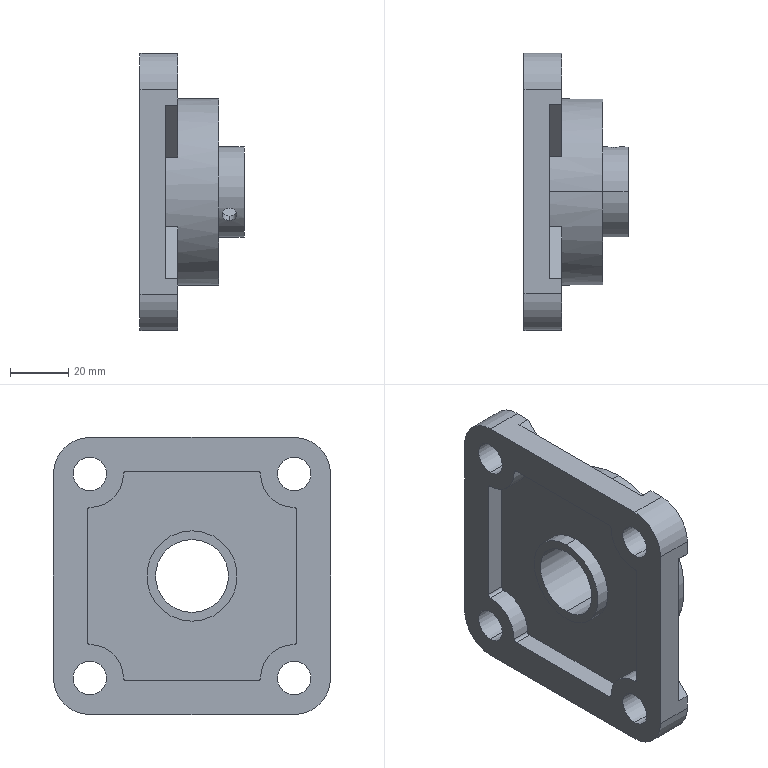Part | SolidWorks | features MBimport 1 | 1 solid | 68 faces | box 35.7 x 95 x 95 mm | volume 103360 mm3 | cylinder 38 | plane 30 | commonest cylinder face diameters 2 x8 11.5 x8 25 x6 4.917 x4 23 x4 31 x4